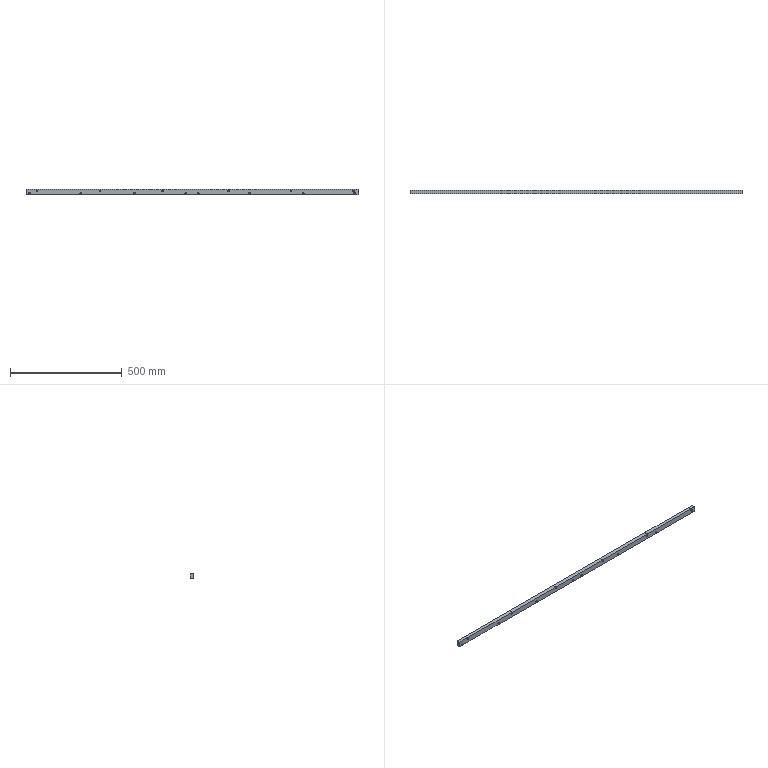Part | STEP file | J013-EBZ05-05-06-Part-1 | 1 solid | 78 faces | box 1485 x 16 x 24 mm | volume 525408 mm3 | cylinder 56 | plane 22 | commonest cylinder face diameters 4.5 x16 8.5 x16 6.8 x12 12 x12